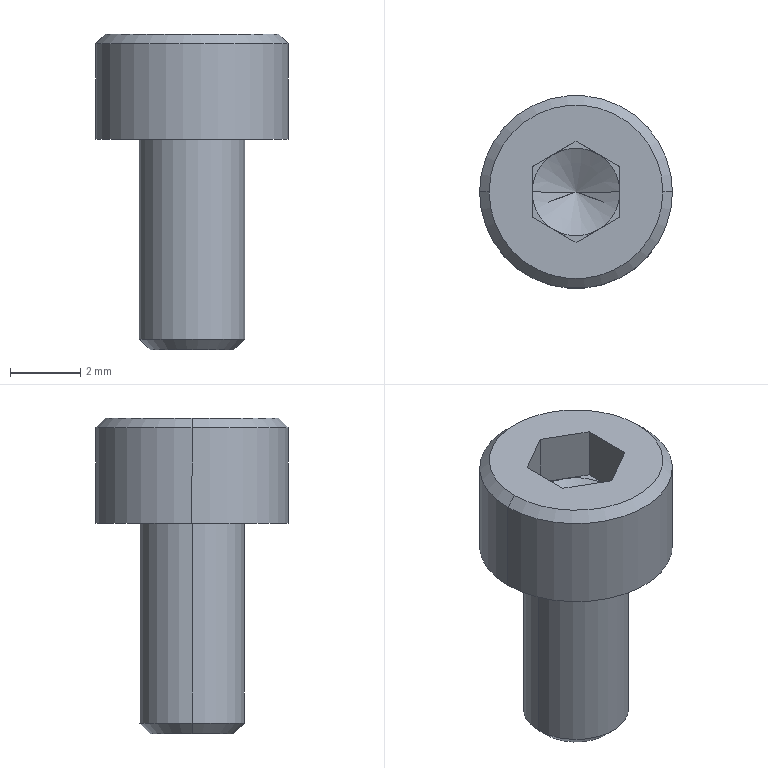Part | NX | features BREP 1 | 1 solid | 25 faces | box 5.5 x 5.5 x 9 mm | volume 103.342 mm3 | plane 15 | cone 6 | cylinder 4 | commonest cylinder face diameters 3 x2 5.5 x2
STEP:
#1=CARTESIAN_POINT('',(0.,0.,0.7783));
#2=VERTEX_POINT('',#1);
#3=CARTESIAN_POINT('',(1.25,0.,1.5));
#4=VERTEX_POINT('',#3);
#5=CARTESIAN_POINT('',(0.,0.,0.7783));
#6=DIRECTION('',(0.866,0.,0.5));
#7=VECTOR('',#6,1000.);
#8=LINE('',#5,#7);
#9=EDGE_CURVE('',#2,#4,#8,.T.);
#10=ORIENTED_EDGE('',*,*,#9,.F.);
#11=CARTESIAN_POINT('',(-1.25,0.,1.5));
#12=VERTEX_POINT('',#11);
#13=CARTESIAN_POINT('',(0.,0.,0.7783));
#14=DIRECTION('',(-0.866,0.,0.5));
#15=VECTOR('',#14,1000.);
#16=LINE('',#13,#15);
#17=EDGE_CURVE('',#2,#12,#16,.T.);
#18=ORIENTED_EDGE('',*,*,#17,.T.);
#19=CARTESIAN_POINT('',(-0.625,-1.083,1.5));
#20=VERTEX_POINT('',#19);
#21=CARTESIAN_POINT('',(0.,0.,1.5));
#22=DIRECTION('',(0.,0.,1.));
#23=DIRECTION('',(1.,0.,0.));
#24=AXIS2_PLACEMENT_3D('',#21,#22,#23);
#25=CIRCLE('',#24,1.25);
#26=EDGE_CURVE('',#12,#20,#25,.T.);
#27=ORIENTED_EDGE('',*,*,#26,.T.);
#28=CARTESIAN_POINT('',(0.625,-1.083,1.5));
#29=VERTEX_POINT('',#28);
#30=CARTESIAN_POINT('',(0.,0.,1.5));
#31=DIRECTION('',(0.,0.,1.));
#32=DIRECTION('',(1.,0.,0.));
#33=AXIS2_PLACEMENT_3D('',#30,#31,#32);
#34=CIRCLE('',#33,1.25);
#35=EDGE_CURVE('',#20,#29,#34,.T.);
#36=ORIENTED_EDGE('',*,*,#35,.T.);
#37=CARTESIAN_POINT('',(0.,0.,1.5));
#38=DIRECTION('',(0.,0.,1.));
#39=DIRECTION('',(1.,0.,0.));
#40=AXIS2_PLACEMENT_3D('',#37,#38,#39);
#41=CIRCLE('',#40,1.25);
#42=EDGE_CURVE('',#29,#4,#41,.T.);
#43=ORIENTED_EDGE('',*,*,#42,.T.);
#44=EDGE_LOOP('',(#10,#18,#27,#36,#43));
#45=FACE_BOUND('',#44,.T.);
#46=CARTESIAN_POINT('',(0.,0.,1000.778));
#47=DIRECTION('',(0.,0.,1.));
#48=DIRECTION('',(-1.,0.,0.));
#49=AXIS2_PLACEMENT_3D('',#46,#47,#48);
#50=CONICAL_SURFACE('',#49,1732.051,1.047);
#51=ADVANCED_FACE('',(#45),#50,.F.);
#52=CARTESIAN_POINT('',(2.75,0.,0.));
#53=VERTEX_POINT('',#52);
#54=CARTESIAN_POINT('',(-2.75,0.,0.));
#55=VERTEX_POINT('',#54);
#56=CARTESIAN_POINT('',(0.,0.,0.));
#57=DIRECTION('',(0.,0.,1.));
#58=DIRECTION('',(1.,0.,0.));
#59=AXIS2_PLACEMENT_3D('',#56,#57,#58);
#60=CIRCLE('',#59,2.75);
#61=EDGE_CURVE('',#53,#55,#60,.T.);
#62=ORIENTED_EDGE('',*,*,#61,.T.);
#63=CARTESIAN_POINT('',(-2.75,0.,2.725));
#64=VERTEX_POINT('',#63);
#65=CARTESIAN_POINT('',(-2.75,0.,0.));
#66=DIRECTION('',(0.,0.,1.));
#67=VECTOR('',#66,1000.);
#68=LINE('',#65,#67);
#69=EDGE_CURVE('',#55,#64,#68,.T.);
#70=ORIENTED_EDGE('',*,*,#69,.T.);
#71=CARTESIAN_POINT('',(2.75,0.,2.725));
#72=VERTEX_POINT('',#71);
#73=CARTESIAN_POINT('',(0.,0.,2.725));
#74=DIRECTION('',(0.,0.,1.));
#75=DIRECTION('',(1.,0.,0.));
#76=AXIS2_PLACEMENT_3D('',#73,#74,#75);
#77=CIRCLE('',#76,2.75);
#78=EDGE_CURVE('',#72,#64,#77,.T.);
#79=ORIENTED_EDGE('',*,*,#78,.F.);
#80=CARTESIAN_POINT('',(2.75,0.,0.));
#81=DIRECTION('',(0.,0.,1.));
#82=VECTOR('',#81,1000.);
#83=LINE('',#80,#82);
#84=EDGE_CURVE('',#53,#72,#83,.T.);
#85=ORIENTED_EDGE('',*,*,#84,.F.);
#86=EDGE_LOOP('',(#62,#70,#79,#85));
#87=FACE_BOUND('',#86,.T.);
#88=CARTESIAN_POINT('',(0.,0.,0.));
#89=DIRECTION('',(0.,0.,1.));
#90=DIRECTION('',(-1.,0.,0.));
#91=AXIS2_PLACEMENT_3D('',#88,#89,#90);
#92=CYLINDRICAL_SURFACE('',#91,2.75);
#93=ADVANCED_FACE('',(#87),#92,.T.);
#94=CARTESIAN_POINT('',(2.475,0.,3.));
#95=VERTEX_POINT('',#94);
#96=CARTESIAN_POINT('',(-2.475,0.,3.));
#97=VERTEX_POINT('',#96);
#98=CARTESIAN_POINT('',(0.,0.,3.));
#99=DIRECTION('',(0.,0.,1.));
#100=DIRECTION('',(1.,0.,0.));
#101=AXIS2_PLACEMENT_3D('',#98,#99,#100);
#102=CIRCLE('',#101,2.475);
#103=EDGE_CURVE('',#95,#97,#102,.T.);
#104=ORIENTED_EDGE('',*,*,#103,.F.);
#105=CARTESIAN_POINT('',(2.75,0.,2.725));
#106=DIRECTION('',(0.7071,0.,-0.7071));
#107=VECTOR('',#106,1000.);
#108=LINE('',#105,#107);
#109=EDGE_CURVE('',#72,#95,#108,.F.);
#110=ORIENTED_EDGE('',*,*,#109,.F.);
#111=ORIENTED_EDGE('',*,*,#78,.T.);
#112=CARTESIAN_POINT('',(-2.75,0.,2.725));
#113=DIRECTION('',(-0.7071,0.,-0.7071));
#114=VECTOR('',#113,1000.);
#115=LINE('',#112,#114);
#116=EDGE_CURVE('',#64,#97,#115,.F.);
#117=ORIENTED_EDGE('',*,*,#116,.T.);
#118=EDGE_LOOP('',(#104,#110,#111,#117));
#119=FACE_BOUND('',#118,.T.);
#120=CARTESIAN_POINT('',(0.,0.,2.725));
#121=DIRECTION('',(0.,0.,-1.));
#122=DIRECTION('',(1.,0.,0.));
#123=AXIS2_PLACEMENT_3D('',#120,#121,#122);
#124=CONICAL_SURFACE('',#123,2.75,0.7854);
#125=ADVANCED_FACE('',(#119),#124,.T.);
#126=CARTESIAN_POINT('',(1.194,0.,-6.));
#127=VERTEX_POINT('',#126);
#128=CARTESIAN_POINT('',(-1.194,0.,-6.));
#129=VERTEX_POINT('',#128);
#130=CARTESIAN_POINT('',(0.,0.,-6.));
#131=DIRECTION('',(0.,0.,1.));
#132=DIRECTION('',(1.,0.,0.));
#133=AXIS2_PLACEMENT_3D('',#130,#131,#132);
#134=CIRCLE('',#133,1.194);
#135=EDGE_CURVE('',#127,#129,#134,.T.);
#136=ORIENTED_EDGE('',*,*,#135,.T.);
#137=CARTESIAN_POINT('',(-1.5,0.,-5.694));
#138=VERTEX_POINT('',#137);
#139=CARTESIAN_POINT('',(-1.194,0.,-6.));
#140=DIRECTION('',(-0.7071,0.,0.7071));
#141=VECTOR('',#140,1000.);
#142=LINE('',#139,#141);
#143=EDGE_CURVE('',#129,#138,#142,.T.);
#144=ORIENTED_EDGE('',*,*,#143,.T.);
#145=CARTESIAN_POINT('',(1.5,0.,-5.694));
#146=VERTEX_POINT('',#145);
#147=CARTESIAN_POINT('',(0.,0.,-5.694));
#148=DIRECTION('',(0.,0.,1.));
#149=DIRECTION('',(1.,0.,0.));
#150=AXIS2_PLACEMENT_3D('',#147,#148,#149);
#151=CIRCLE('',#150,1.5);
#152=EDGE_CURVE('',#146,#138,#151,.T.);
#153=ORIENTED_EDGE('',*,*,#152,.F.);
#154=CARTESIAN_POINT('',(1.194,0.,-6.));
#155=DIRECTION('',(0.7071,0.,0.7071));
#156=VECTOR('',#155,1000.);
#157=LINE('',#154,#156);
#158=EDGE_CURVE('',#127,#146,#157,.T.);
#159=ORIENTED_EDGE('',*,*,#158,.F.);
#160=EDGE_LOOP('',(#136,#144,#153,#159));
#161=FACE_BOUND('',#160,.T.);
#162=CARTESIAN_POINT('',(0.,0.,-6.));
#163=DIRECTION('',(0.,0.,1.));
#164=DIRECTION('',(-1.,0.,0.));
#165=AXIS2_PLACEMENT_3D('',#162,#163,#164);
#166=CONICAL_SURFACE('',#165,1.194,0.7854);
#167=ADVANCED_FACE('',(#161),#166,.T.);
#168=ORIENTED_EDGE('',*,*,#152,.T.);
#169=CARTESIAN_POINT('',(-1.5,0.,0.));
#170=VERTEX_POINT('',#169);
#171=CARTESIAN_POINT('',(-1.5,0.,-6.));
#172=DIRECTION('',(0.,0.,1.));
#173=VECTOR('',#172,1000.);
#174=LINE('',#171,#173);
#175=EDGE_CURVE('',#138,#170,#174,.T.);
#176=ORIENTED_EDGE('',*,*,#175,.T.);
#177=CARTESIAN_POINT('',(1.5,0.,0.));
#178=VERTEX_POINT('',#177);
#179=CARTESIAN_POINT('',(0.,0.,0.));
#180=DIRECTION('',(0.,0.,1.));
#181=DIRECTION('',(1.,0.,0.));
#182=AXIS2_PLACEMENT_3D('',#179,#180,#181);
#183=CIRCLE('',#182,1.5);
#184=EDGE_CURVE('',#178,#170,#183,.T.);
#185=ORIENTED_EDGE('',*,*,#184,.F.);
#186=CARTESIAN_POINT('',(1.5,0.,-6.));
#187=DIRECTION('',(0.,0.,1.));
#188=VECTOR('',#187,1000.);
#189=LINE('',#186,#188);
#190=EDGE_CURVE('',#146,#178,#189,.T.);
#191=ORIENTED_EDGE('',*,*,#190,.F.);
#192=EDGE_LOOP('',(#168,#176,#185,#191));
#193=FACE_BOUND('',#192,.T.);
#194=CARTESIAN_POINT('',(0.,0.,-6.));
#195=DIRECTION('',(0.,0.,1.));
#196=DIRECTION('',(-1.,0.,0.));
#197=AXIS2_PLACEMENT_3D('',#194,#195,#196);
#198=CYLINDRICAL_SURFACE('',#197,1.5);
#199=ADVANCED_FACE('',(#193),#198,.T.);
#200=CARTESIAN_POINT('',(0.625,1.083,1.5));
#201=VERTEX_POINT('',#200);
#202=CARTESIAN_POINT('',(0.,0.,1.5));
#203=DIRECTION('',(0.,0.,1.));
#204=DIRECTION('',(1.,0.,0.));
#205=AXIS2_PLACEMENT_3D('',#202,#203,#204);
#206=CIRCLE('',#205,1.25);
#207=EDGE_CURVE('',#4,#201,#206,.T.);
#208=ORIENTED_EDGE('',*,*,#207,.F.);
#209=CARTESIAN_POINT('',(1.25,0.7217,1.5));
#210=VERTEX_POINT('',#209);
#211=CARTESIAN_POINT('',(1.25,-0.7217,1.5));
#212=DIRECTION('',(0.,1.,0.));
#213=VECTOR('',#212,1000.);
#214=LINE('',#211,#213);
#215=EDGE_CURVE('',#4,#210,#214,.T.);
#216=ORIENTED_EDGE('',*,*,#215,.T.);
#217=CARTESIAN_POINT('',(1.25,0.7217,1.5));
#218=DIRECTION('',(-0.866,0.5,0.));
#219=VECTOR('',#218,1000.);
#220=LINE('',#217,#219);
#221=EDGE_CURVE('',#210,#201,#220,.T.);
#222=ORIENTED_EDGE('',*,*,#221,.T.);
#223=EDGE_LOOP('',(#208,#216,#222));
#224=FACE_BOUND('',#223,.T.);
#225=CARTESIAN_POINT('',(0.,0.,1.5));
#226=DIRECTION('',(0.,0.,1.));
#227=DIRECTION('',(-1.,0.,0.));
#228=AXIS2_PLACEMENT_3D('',#225,#226,#227);
#229=PLANE('',#228);
#230=ADVANCED_FACE('',(#224),#229,.T.);
#231=CARTESIAN_POINT('',(-0.625,1.083,1.5));
#232=VERTEX_POINT('',#231);
#233=CARTESIAN_POINT('',(0.,0.,1.5));
#234=DIRECTION('',(0.,0.,1.));
#235=DIRECTION('',(1.,0.,0.));
#236=AXIS2_PLACEMENT_3D('',#233,#234,#235);
#237=CIRCLE('',#236,1.25);
#238=EDGE_CURVE('',#201,#232,#237,.T.);
#239=ORIENTED_EDGE('',*,*,#238,.F.);
#240=CARTESIAN_POINT('',(0.,1.443,1.5));
#241=VERTEX_POINT('',#240);
#242=CARTESIAN_POINT('',(1.25,0.7217,1.5));
#243=DIRECTION('',(-0.866,0.5,0.));
#244=VECTOR('',#243,1000.);
#245=LINE('',#242,#244);
#246=EDGE_CURVE('',#201,#241,#245,.T.);
#247=ORIENTED_EDGE('',*,*,#246,.T.);
#248=CARTESIAN_POINT('',(0.,1.443,1.5));
#249=DIRECTION('',(-0.866,-0.5,0.));
#250=VECTOR('',#249,1000.);
#251=LINE('',#248,#250);
#252=EDGE_CURVE('',#241,#232,#251,.T.);
#253=ORIENTED_EDGE('',*,*,#252,.T.);
#254=EDGE_LOOP('',(#239,#247,#253));
#255=FACE_BOUND('',#254,.T.);
#256=CARTESIAN_POINT('',(0.,0.,1.5));
#257=DIRECTION('',(0.,0.,1.));
#258=DIRECTION('',(-1.,0.,0.));
#259=AXIS2_PLACEMENT_3D('',#256,#257,#258);
#260=PLANE('',#259);
#261=ADVANCED_FACE('',(#255),#260,.T.);
#262=CARTESIAN_POINT('',(0.,0.,1.5));
#263=DIRECTION('',(0.,0.,1.));
#264=DIRECTION('',(1.,0.,0.));
#265=AXIS2_PLACEMENT_3D('',#262,#263,#264);
#266=CIRCLE('',#265,1.25);
#267=EDGE_CURVE('',#232,#12,#266,.T.);
#268=ORIENTED_EDGE('',*,*,#267,.F.);
#269=CARTESIAN_POINT('',(-1.25,0.7217,1.5));
#270=VERTEX_POINT('',#269);
#271=CARTESIAN_POINT('',(0.,1.443,1.5));
#272=DIRECTION('',(-0.866,-0.5,0.));
#273=VECTOR('',#272,1000.);
#274=LINE('',#271,#273);
#275=EDGE_CURVE('',#232,#270,#274,.T.);
#276=ORIENTED_EDGE('',*,*,#275,.T.);
#277=CARTESIAN_POINT('',(-1.25,0.7217,1.5));
#278=DIRECTION('',(0.,-1.,0.));
#279=VECTOR('',#278,1000.);
#280=LINE('',#277,#279);
#281=EDGE_CURVE('',#270,#12,#280,.T.);
#282=ORIENTED_EDGE('',*,*,#281,.T.);
#283=EDGE_LOOP('',(#268,#276,#282));
#284=FACE_BOUND('',#283,.T.);
#285=CARTESIAN_POINT('',(0.,0.,1.5));
#286=DIRECTION('',(0.,0.,1.));
#287=DIRECTION('',(-1.,0.,0.));
#288=AXIS2_PLACEMENT_3D('',#285,#286,#287);
#289=PLANE('',#288);
#290=ADVANCED_FACE('',(#284),#289,.T.);
#291=ORIENTED_EDGE('',*,*,#26,.F.);
#292=CARTESIAN_POINT('',(-1.25,-0.7217,1.5));
#293=VERTEX_POINT('',#292);
#294=CARTESIAN_POINT('',(-1.25,0.7217,1.5));
#295=DIRECTION('',(0.,-1.,0.));
#296=VECTOR('',#295,1000.);
#297=LINE('',#294,#296);
#298=EDGE_CURVE('',#12,#293,#297,.T.);
#299=ORIENTED_EDGE('',*,*,#298,.T.);
#300=CARTESIAN_POINT('',(-1.25,-0.7217,1.5));
#301=DIRECTION('',(0.866,-0.5,0.));
#302=VECTOR('',#301,1000.);
#303=LINE('',#300,#302);
#304=EDGE_CURVE('',#293,#20,#303,.T.);
#305=ORIENTED_EDGE('',*,*,#304,.T.);
#306=EDGE_LOOP('',(#291,#299,#305));
#307=FACE_BOUND('',#306,.T.);
#308=CARTESIAN_POINT('',(0.,0.,1.5));
#309=DIRECTION('',(0.,0.,1.));
#310=DIRECTION('',(-1.,0.,0.));
#311=AXIS2_PLACEMENT_3D('',#308,#309,#310);
#312=PLANE('',#311);
#313=ADVANCED_FACE('',(#307),#312,.T.);
#314=ORIENTED_EDGE('',*,*,#35,.F.);
#315=CARTESIAN_POINT('',(0.,-1.443,1.5));
#316=VERTEX_POINT('',#315);
#317=CARTESIAN_POINT('',(-1.25,-0.7217,1.5));
#318=DIRECTION('',(0.866,-0.5,0.));
#319=VECTOR('',#318,1000.);
#320=LINE('',#317,#319);
#321=EDGE_CURVE('',#20,#316,#320,.T.);
#322=ORIENTED_EDGE('',*,*,#321,.T.);
#323=CARTESIAN_POINT('',(0.,-1.443,1.5));
#324=DIRECTION('',(0.866,0.5,0.));
#325=VECTOR('',#324,1000.);
#326=LINE('',#323,#325);
#327=EDGE_CURVE('',#316,#29,#326,.T.);
#328=ORIENTED_EDGE('',*,*,#327,.T.);
#329=EDGE_LOOP('',(#314,#322,#328));
#330=FACE_BOUND('',#329,.T.);
#331=CARTESIAN_POINT('',(0.,0.,1.5));
#332=DIRECTION('',(0.,0.,1.));
#333=DIRECTION('',(-1.,0.,0.));
#334=AXIS2_PLACEMENT_3D('',#331,#332,#333);
#335=PLANE('',#334);
#336=ADVANCED_FACE('',(#330),#335,.T.);
#337=ORIENTED_EDGE('',*,*,#175,.F.);
#338=CARTESIAN_POINT('',(0.,0.,-5.694));
#339=DIRECTION('',(0.,0.,1.));
#340=DIRECTION('',(1.,0.,0.));
#341=AXIS2_PLACEMENT_3D('',#338,#339,#340);
#342=CIRCLE('',#341,1.5);
#343=EDGE_CURVE('',#138,#146,#342,.T.);
#344=ORIENTED_EDGE('',*,*,#343,.T.);
#345=ORIENTED_EDGE('',*,*,#190,.T.);
#346=CARTESIAN_POINT('',(0.,0.,0.));
#347=DIRECTION('',(0.,0.,1.));
#348=DIRECTION('',(1.,0.,0.));
#349=AXIS2_PLACEMENT_3D('',#346,#347,#348);
#350=CIRCLE('',#349,1.5);
#351=EDGE_CURVE('',#170,#178,#350,.T.);
#352=ORIENTED_EDGE('',*,*,#351,.F.);
#353=EDGE_LOOP('',(#337,#344,#345,#352));
#354=FACE_BOUND('',#353,.T.);
#355=CARTESIAN_POINT('',(0.,0.,-6.));
#356=DIRECTION('',(0.,0.,1.));
#357=DIRECTION('',(-1.,0.,0.));
#358=AXIS2_PLACEMENT_3D('',#355,#356,#357);
#359=CYLINDRICAL_SURFACE('',#358,1.5);
#360=ADVANCED_FACE('',(#354),#359,.T.);
#361=ORIENTED_EDGE('',*,*,#143,.F.);
#362=CARTESIAN_POINT('',(0.,0.,-6.));
#363=DIRECTION('',(0.,0.,1.));
#364=DIRECTION('',(1.,0.,0.));
#365=AXIS2_PLACEMENT_3D('',#362,#363,#364);
#366=CIRCLE('',#365,1.194);
#367=EDGE_CURVE('',#129,#127,#366,.T.);
#368=ORIENTED_EDGE('',*,*,#367,.T.);
#369=ORIENTED_EDGE('',*,*,#158,.T.);
#370=ORIENTED_EDGE('',*,*,#343,.F.);
#371=EDGE_LOOP('',(#361,#368,#369,#370));
#372=FACE_BOUND('',#371,.T.);
#373=CARTESIAN_POINT('',(0.,0.,-6.));
#374=DIRECTION('',(0.,0.,1.));
#375=DIRECTION('',(-1.,0.,0.));
#376=AXIS2_PLACEMENT_3D('',#373,#374,#375);
#377=CONICAL_SURFACE('',#376,1.194,0.7854);
#378=ADVANCED_FACE('',(#372),#377,.T.);
#379=ORIENTED_EDGE('',*,*,#135,.F.);
#380=ORIENTED_EDGE('',*,*,#367,.F.);
#381=EDGE_LOOP('',(#379,#380));
#382=FACE_BOUND('',#381,.T.);
#383=CARTESIAN_POINT('',(0.,1.194,-6.));
#384=DIRECTION('',(0.,0.,1.));
#385=DIRECTION('',(-1.,0.,0.));
#386=AXIS2_PLACEMENT_3D('',#383,#384,#385);
#387=PLANE('',#386);
#388=ADVANCED_FACE('',(#382),#387,.F.);
#389=CARTESIAN_POINT('',(0.,-1.443,3.));
#390=VERTEX_POINT('',#389);
#391=CARTESIAN_POINT('',(1.25,-0.7217,3.));
#392=VERTEX_POINT('',#391);
#393=CARTESIAN_POINT('',(0.,-1.443,3.));
#394=DIRECTION('',(0.866,0.5,0.));
#395=VECTOR('',#394,1000.);
#396=LINE('',#393,#395);
#397=EDGE_CURVE('',#390,#392,#396,.T.);
#398=ORIENTED_EDGE('',*,*,#397,.F.);
#399=CARTESIAN_POINT('',(-1.25,-0.7217,3.));
#400=VERTEX_POINT('',#399);
#401=CARTESIAN_POINT('',(-1.25,-0.7217,3.));
#402=DIRECTION('',(0.866,-0.5,0.));
#403=VECTOR('',#402,1000.);
#404=LINE('',#401,#403);
#405=EDGE_CURVE('',#400,#390,#404,.T.);
#406=ORIENTED_EDGE('',*,*,#405,.F.);
#407=CARTESIAN_POINT('',(-1.25,0.7217,3.));
#408=VERTEX_POINT('',#407);
#409=CARTESIAN_POINT('',(-1.25,0.7217,3.));
#410=DIRECTION('',(0.,-1.,0.));
#411=VECTOR('',#410,1000.);
#412=LINE('',#409,#411);
#413=EDGE_CURVE('',#408,#400,#412,.T.);
#414=ORIENTED_EDGE('',*,*,#413,.F.);
#415=CARTESIAN_POINT('',(0.,1.443,3.));
#416=VERTEX_POINT('',#415);
#417=CARTESIAN_POINT('',(0.,1.443,3.));
#418=DIRECTION('',(-0.866,-0.5,0.));
#419=VECTOR('',#418,1000.);
#420=LINE('',#417,#419);
#421=EDGE_CURVE('',#416,#408,#420,.T.);
#422=ORIENTED_EDGE('',*,*,#421,.F.);
#423=CARTESIAN_POINT('',(1.25,0.7217,3.));
#424=VERTEX_POINT('',#423);
#425=CARTESIAN_POINT('',(1.25,0.7217,3.));
#426=DIRECTION('',(-0.866,0.5,0.));
#427=VECTOR('',#426,1000.);
#428=LINE('',#425,#427);
#429=EDGE_CURVE('',#424,#416,#428,.T.);
#430=ORIENTED_EDGE('',*,*,#429,.F.);
#431=CARTESIAN_POINT('',(1.25,-0.7217,3.));
#432=DIRECTION('',(0.,1.,0.));
#433=VECTOR('',#432,1000.);
#434=LINE('',#431,#433);
#435=EDGE_CURVE('',#392,#424,#434,.T.);
#436=ORIENTED_EDGE('',*,*,#435,.F.);
#437=EDGE_LOOP('',(#398,#406,#414,#422,#430,#436));
#438=FACE_BOUND('',#437,.T.);
#439=CARTESIAN_POINT('',(0.,0.,3.));
#440=DIRECTION('',(0.,0.,1.));
#441=DIRECTION('',(1.,0.,0.));
#442=AXIS2_PLACEMENT_3D('',#439,#440,#441);
#443=CIRCLE('',#442,2.475);
#444=EDGE_CURVE('',#97,#95,#443,.T.);
#445=ORIENTED_EDGE('',*,*,#444,.T.);
#446=ORIENTED_EDGE('',*,*,#103,.T.);
#447=EDGE_LOOP('',(#445,#446));
#448=FACE_BOUND('',#447,.T.);
#449=CARTESIAN_POINT('',(0.,0.,3.));
#450=DIRECTION('',(0.,0.,-1.));
#451=DIRECTION('',(1.,0.,0.));
#452=AXIS2_PLACEMENT_3D('',#449,#450,#451);
#453=PLANE('',#452);
#454=ADVANCED_FACE('',(#438,#448),#453,.F.);
#455=ORIENTED_EDGE('',*,*,#109,.T.);
#456=ORIENTED_EDGE('',*,*,#444,.F.);
#457=ORIENTED_EDGE('',*,*,#116,.F.);
#458=CARTESIAN_POINT('',(0.,0.,2.725));
#459=DIRECTION('',(0.,0.,1.));
#460=DIRECTION('',(1.,0.,0.));
#461=AXIS2_PLACEMENT_3D('',#458,#459,#460);
#462=CIRCLE('',#461,2.75);
#463=EDGE_CURVE('',#64,#72,#462,.T.);
#464=ORIENTED_EDGE('',*,*,#463,.T.);
#465=EDGE_LOOP('',(#455,#456,#457,#464));
#466=FACE_BOUND('',#465,.T.);
#467=CARTESIAN_POINT('',(0.,0.,2.725));
#468=DIRECTION('',(0.,0.,-1.));
#469=DIRECTION('',(1.,0.,0.));
#470=AXIS2_PLACEMENT_3D('',#467,#468,#469);
#471=CONICAL_SURFACE('',#470,2.75,0.7854);
#472=ADVANCED_FACE('',(#466),#471,.T.);
#473=ORIENTED_EDGE('',*,*,#69,.F.);
#474=CARTESIAN_POINT('',(0.,0.,0.));
#475=DIRECTION('',(0.,0.,1.));
#476=DIRECTION('',(1.,0.,0.));
#477=AXIS2_PLACEMENT_3D('',#474,#475,#476);
#478=CIRCLE('',#477,2.75);
#479=EDGE_CURVE('',#55,#53,#478,.T.);
#480=ORIENTED_EDGE('',*,*,#479,.T.);
#481=ORIENTED_EDGE('',*,*,#84,.T.);
#482=ORIENTED_EDGE('',*,*,#463,.F.);
#483=EDGE_LOOP('',(#473,#480,#481,#482));
#484=FACE_BOUND('',#483,.T.);
#485=CARTESIAN_POINT('',(0.,0.,0.));
#486=DIRECTION('',(0.,0.,1.));
#487=DIRECTION('',(-1.,0.,0.));
#488=AXIS2_PLACEMENT_3D('',#485,#486,#487);
#489=CYLINDRICAL_SURFACE('',#488,2.75);
#490=ADVANCED_FACE('',(#484),#489,.T.);
#491=ORIENTED_EDGE('',*,*,#184,.T.);
#492=ORIENTED_EDGE('',*,*,#351,.T.);
#493=EDGE_LOOP('',(#491,#492));
#494=FACE_BOUND('',#493,.T.);
#495=ORIENTED_EDGE('',*,*,#61,.F.);
#496=ORIENTED_EDGE('',*,*,#479,.F.);
#497=EDGE_LOOP('',(#495,#496));
#498=FACE_BOUND('',#497,.T.);
#499=CARTESIAN_POINT('',(0.,2.75,0.));
#500=DIRECTION('',(0.,0.,1.));
#501=DIRECTION('',(-1.,0.,0.));
#502=AXIS2_PLACEMENT_3D('',#499,#500,#501);
#503=PLANE('',#502);
#504=ADVANCED_FACE('',(#494,#498),#503,.F.);
#505=ORIENTED_EDGE('',*,*,#405,.T.);
#506=CARTESIAN_POINT('',(0.,-1.443,1.5));
#507=DIRECTION('',(0.,0.,1.));
#508=VECTOR('',#507,1000.);
#509=LINE('',#506,#508);
#510=EDGE_CURVE('',#316,#390,#509,.T.);
#511=ORIENTED_EDGE('',*,*,#510,.F.);
#512=ORIENTED_EDGE('',*,*,#321,.F.);
#513=ORIENTED_EDGE('',*,*,#304,.F.);
#514=CARTESIAN_POINT('',(-1.25,-0.7217,1.5));
#515=DIRECTION('',(0.,0.,1.));
#516=VECTOR('',#515,1000.);
#517=LINE('',#514,#516);
#518=EDGE_CURVE('',#293,#400,#517,.T.);
#519=ORIENTED_EDGE('',*,*,#518,.T.);
#520=EDGE_LOOP('',(#505,#511,#512,#513,#519));
#521=FACE_BOUND('',#520,.T.);
#522=CARTESIAN_POINT('',(-1.25,-0.7217,1.5));
#523=DIRECTION('',(-0.5,-0.866,0.));
#524=DIRECTION('',(-0.866,0.5,0.));
#525=AXIS2_PLACEMENT_3D('',#522,#523,#524);
#526=PLANE('',#525);
#527=ADVANCED_FACE('',(#521),#526,.F.);
#528=ORIENTED_EDGE('',*,*,#413,.T.);
#529=ORIENTED_EDGE('',*,*,#518,.F.);
#530=ORIENTED_EDGE('',*,*,#298,.F.);
#531=ORIENTED_EDGE('',*,*,#281,.F.);
#532=CARTESIAN_POINT('',(-1.25,0.7217,1.5));
#533=DIRECTION('',(0.,0.,1.));
#534=VECTOR('',#533,1000.);
#535=LINE('',#532,#534);
#536=EDGE_CURVE('',#270,#408,#535,.T.);
#537=ORIENTED_EDGE('',*,*,#536,.T.);
#538=EDGE_LOOP('',(#528,#529,#530,#531,#537));
#539=FACE_BOUND('',#538,.T.);
#540=CARTESIAN_POINT('',(-1.25,0.7217,1.5));
#541=DIRECTION('',(-1.,0.,0.));
#542=DIRECTION('',(0.,0.,-1.));
#543=AXIS2_PLACEMENT_3D('',#540,#541,#542);
#544=PLANE('',#543);
#545=ADVANCED_FACE('',(#539),#544,.F.);
#546=ORIENTED_EDGE('',*,*,#421,.T.);
#547=ORIENTED_EDGE('',*,*,#536,.F.);
#548=ORIENTED_EDGE('',*,*,#275,.F.);
#549=ORIENTED_EDGE('',*,*,#252,.F.);
#550=CARTESIAN_POINT('',(0.,1.443,1.5));
#551=DIRECTION('',(0.,0.,1.));
#552=VECTOR('',#551,1000.);
#553=LINE('',#550,#552);
#554=EDGE_CURVE('',#241,#416,#553,.T.);
#555=ORIENTED_EDGE('',*,*,#554,.T.);
#556=EDGE_LOOP('',(#546,#547,#548,#549,#555));
#557=FACE_BOUND('',#556,.T.);
#558=CARTESIAN_POINT('',(0.,1.443,1.5));
#559=DIRECTION('',(-0.5,0.866,0.));
#560=DIRECTION('',(0.866,0.5,0.));
#561=AXIS2_PLACEMENT_3D('',#558,#559,#560);
#562=PLANE('',#561);
#563=ADVANCED_FACE('',(#557),#562,.F.);
#564=ORIENTED_EDGE('',*,*,#429,.T.);
#565=ORIENTED_EDGE('',*,*,#554,.F.);
#566=ORIENTED_EDGE('',*,*,#246,.F.);
#567=ORIENTED_EDGE('',*,*,#221,.F.);
#568=CARTESIAN_POINT('',(1.25,0.7217,1.5));
#569=DIRECTION('',(0.,0.,1.));
#570=VECTOR('',#569,1000.);
#571=LINE('',#568,#570);
#572=EDGE_CURVE('',#210,#424,#571,.T.);
#573=ORIENTED_EDGE('',*,*,#572,.T.);
#574=EDGE_LOOP('',(#564,#565,#566,#567,#573));
#575=FACE_BOUND('',#574,.T.);
#576=CARTESIAN_POINT('',(1.25,0.7217,1.5));
#577=DIRECTION('',(0.5,0.866,0.));
#578=DIRECTION('',(0.866,-0.5,0.));
#579=AXIS2_PLACEMENT_3D('',#576,#577,#578);
#580=PLANE('',#579);
#581=ADVANCED_FACE('',(#575),#580,.F.);
#582=ORIENTED_EDGE('',*,*,#435,.T.);
#583=ORIENTED_EDGE('',*,*,#572,.F.);
#584=ORIENTED_EDGE('',*,*,#215,.F.);
#585=CARTESIAN_POINT('',(1.25,-0.7217,1.5));
#586=VERTEX_POINT('',#585);
#587=CARTESIAN_POINT('',(1.25,-0.7217,1.5));
#588=DIRECTION('',(0.,1.,0.));
#589=VECTOR('',#588,1000.);
#590=LINE('',#587,#589);
#591=EDGE_CURVE('',#586,#4,#590,.T.);
#592=ORIENTED_EDGE('',*,*,#591,.F.);
#593=CARTESIAN_POINT('',(1.25,-0.7217,1.5));
#594=DIRECTION('',(0.,0.,1.));
#595=VECTOR('',#594,1000.);
#596=LINE('',#593,#595);
#597=EDGE_CURVE('',#586,#392,#596,.T.);
#598=ORIENTED_EDGE('',*,*,#597,.T.);
#599=EDGE_LOOP('',(#582,#583,#584,#592,#598));
#600=FACE_BOUND('',#599,.T.);
#601=CARTESIAN_POINT('',(1.25,-0.7217,1.5));
#602=DIRECTION('',(1.,0.,0.));
#603=DIRECTION('',(0.,0.,1.));
#604=AXIS2_PLACEMENT_3D('',#601,#602,#603);
#605=PLANE('',#604);
#606=ADVANCED_FACE('',(#600),#605,.F.);
#607=ORIENTED_EDGE('',*,*,#397,.T.);
#608=ORIENTED_EDGE('',*,*,#597,.F.);
#609=CARTESIAN_POINT('',(0.,-1.443,1.5));
#610=DIRECTION('',(0.866,0.5,0.));
#611=VECTOR('',#610,1000.);
#612=LINE('',#609,#611);
#613=EDGE_CURVE('',#29,#586,#612,.T.);
#614=ORIENTED_EDGE('',*,*,#613,.F.);
#615=ORIENTED_EDGE('',*,*,#327,.F.);
#616=ORIENTED_EDGE('',*,*,#510,.T.);
#617=EDGE_LOOP('',(#607,#608,#614,#615,#616));
#618=FACE_BOUND('',#617,.T.);
#619=CARTESIAN_POINT('',(0.,-1.443,1.5));
#620=DIRECTION('',(0.5,-0.866,0.));
#621=DIRECTION('',(-0.866,-0.5,0.));
#622=AXIS2_PLACEMENT_3D('',#619,#620,#621);
#623=PLANE('',#622);
#624=ADVANCED_FACE('',(#618),#623,.F.);
#625=ORIENTED_EDGE('',*,*,#42,.F.);
#626=ORIENTED_EDGE('',*,*,#613,.T.);
#627=ORIENTED_EDGE('',*,*,#591,.T.);
#628=EDGE_LOOP('',(#625,#626,#627));
#629=FACE_BOUND('',#628,.T.);
#630=CARTESIAN_POINT('',(0.,0.,1.5));
#631=DIRECTION('',(0.,0.,1.));
#632=DIRECTION('',(-1.,0.,0.));
#633=AXIS2_PLACEMENT_3D('',#630,#631,#632);
#634=PLANE('',#633);
#635=ADVANCED_FACE('',(#629),#634,.T.);
#636=ORIENTED_EDGE('',*,*,#17,.F.);
#637=ORIENTED_EDGE('',*,*,#9,.T.);
#638=ORIENTED_EDGE('',*,*,#207,.T.);
#639=ORIENTED_EDGE('',*,*,#238,.T.);
#640=ORIENTED_EDGE('',*,*,#267,.T.);
#641=EDGE_LOOP('',(#636,#637,#638,#639,#640));
#642=FACE_BOUND('',#641,.T.);
#643=CARTESIAN_POINT('',(0.,0.,1000.778));
#644=DIRECTION('',(0.,0.,1.));
#645=DIRECTION('',(-1.,0.,0.));
#646=AXIS2_PLACEMENT_3D('',#643,#644,#645);
#647=CONICAL_SURFACE('',#646,1732.051,1.047);
#648=ADVANCED_FACE('',(#642),#647,.F.);
#649=CLOSED_SHELL('',(#51,#93,#125,#167,#199,#230,#261,#290,#313,#336,#360,#378,#388,#454,#472,#490,#504,#527,#545,#563,#581,#606,#624,#635,#648));
#650=MANIFOLD_SOLID_BREP('',#649);
#651=(LENGTH_UNIT()NAMED_UNIT(*)SI_UNIT(.MILLI.,.METRE.));
#652=UNCERTAINTY_MEASURE_WITH_UNIT(LENGTH_MEASURE(0.00001),#651,'','');
#653=(NAMED_UNIT(*)PLANE_ANGLE_UNIT()SI_UNIT($,.RADIAN.));
#654=(NAMED_UNIT(*)SI_UNIT($,.STERADIAN.)SOLID_ANGLE_UNIT());
#655=(GEOMETRIC_REPRESENTATION_CONTEXT(3)GLOBAL_UNCERTAINTY_ASSIGNED_CONTEXT((#652))GLOBAL_UNIT_ASSIGNED_CONTEXT((#651,#653,#654))REPRESENTATION_CONTEXT('',''));
#656=ADVANCED_BREP_SHAPE_REPRESENTATION('',(#650),#655);